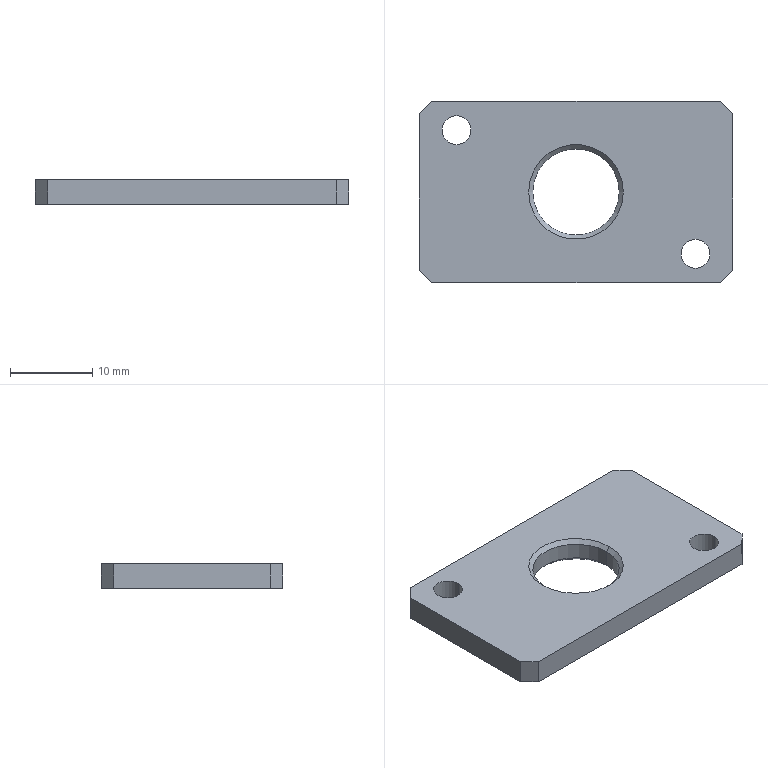Part | SolidWorks | features Chamfer 2, Extrusion 1 | 1 solid | 20 faces | box 38 x 22 x 3 mm | volume 2168 mm3 | plane 10 | cylinder 6 | cone 4 | commonest cylinder face diameters 3.5 x4 10.5 x2
STEP:
#1=CARTESIAN_POINT('',(-5.25,0.,2.5));
#2=VERTEX_POINT('',#1);
#3=CARTESIAN_POINT('',(5.25,0.,2.5));
#4=VERTEX_POINT('',#3);
#5=CARTESIAN_POINT('',(0.,0.,2.5));
#6=DIRECTION('',(0.,0.,1.));
#7=DIRECTION('',(1.,0.,0.));
#8=AXIS2_PLACEMENT_3D('',#5,#6,#7);
#9=CIRCLE('',#8,5.25);
#10=EDGE_CURVE('',#2,#4,#9,.T.);
#11=ORIENTED_EDGE('',*,*,#10,.F.);
#12=CARTESIAN_POINT('',(-5.75,0.,3.));
#13=VERTEX_POINT('',#12);
#14=CARTESIAN_POINT('',(-5.25,0.,2.5));
#15=DIRECTION('',(-0.7071,0.,0.7071));
#16=VECTOR('',#15,1000.);
#17=LINE('',#14,#16);
#18=EDGE_CURVE('',#2,#13,#17,.T.);
#19=ORIENTED_EDGE('',*,*,#18,.T.);
#20=CARTESIAN_POINT('',(5.75,0.,3.));
#21=VERTEX_POINT('',#20);
#22=CARTESIAN_POINT('',(0.,0.,3.));
#23=DIRECTION('',(0.,0.,-1.));
#24=DIRECTION('',(1.,0.,0.));
#25=AXIS2_PLACEMENT_3D('',#22,#23,#24);
#26=CIRCLE('',#25,5.75);
#27=EDGE_CURVE('',#21,#13,#26,.T.);
#28=ORIENTED_EDGE('',*,*,#27,.F.);
#29=CARTESIAN_POINT('',(5.25,0.,2.5));
#30=DIRECTION('',(0.7071,0.,0.7071));
#31=VECTOR('',#30,1000.);
#32=LINE('',#29,#31);
#33=EDGE_CURVE('',#4,#21,#32,.T.);
#34=ORIENTED_EDGE('',*,*,#33,.F.);
#35=EDGE_LOOP('',(#11,#19,#28,#34));
#36=FACE_OUTER_BOUND('',#35,.T.);
#37=CARTESIAN_POINT('',(0.,0.,2.5));
#38=DIRECTION('',(0.,0.,1.));
#39=DIRECTION('',(1.,0.,0.));
#40=AXIS2_PLACEMENT_3D('',#37,#38,#39);
#41=CONICAL_SURFACE('',#40,5.25,0.7854);
#42=ADVANCED_FACE('',(#36),#41,.F.);
#43=CARTESIAN_POINT('',(5.25,0.,0.5));
#44=VERTEX_POINT('',#43);
#45=CARTESIAN_POINT('',(-5.25,0.,0.5));
#46=VERTEX_POINT('',#45);
#47=CARTESIAN_POINT('',(0.,0.,0.5));
#48=DIRECTION('',(0.,0.,-1.));
#49=DIRECTION('',(1.,0.,0.));
#50=AXIS2_PLACEMENT_3D('',#47,#48,#49);
#51=CIRCLE('',#50,5.25);
#52=EDGE_CURVE('',#44,#46,#51,.T.);
#53=ORIENTED_EDGE('',*,*,#52,.F.);
#54=CARTESIAN_POINT('',(5.75,0.,0.));
#55=VERTEX_POINT('',#54);
#56=CARTESIAN_POINT('',(5.75,0.,0.));
#57=DIRECTION('',(0.7071,0.,-0.7071));
#58=VECTOR('',#57,1000.);
#59=LINE('',#56,#58);
#60=EDGE_CURVE('',#44,#55,#59,.T.);
#61=ORIENTED_EDGE('',*,*,#60,.T.);
#62=CARTESIAN_POINT('',(-5.75,0.,0.));
#63=VERTEX_POINT('',#62);
#64=CARTESIAN_POINT('',(0.,0.,0.));
#65=DIRECTION('',(0.,0.,1.));
#66=DIRECTION('',(1.,0.,0.));
#67=AXIS2_PLACEMENT_3D('',#64,#65,#66);
#68=CIRCLE('',#67,5.75);
#69=EDGE_CURVE('',#63,#55,#68,.T.);
#70=ORIENTED_EDGE('',*,*,#69,.F.);
#71=CARTESIAN_POINT('',(-5.75,0.,0.));
#72=DIRECTION('',(-0.7071,0.,-0.7071));
#73=VECTOR('',#72,1000.);
#74=LINE('',#71,#73);
#75=EDGE_CURVE('',#46,#63,#74,.T.);
#76=ORIENTED_EDGE('',*,*,#75,.F.);
#77=EDGE_LOOP('',(#53,#61,#70,#76));
#78=FACE_OUTER_BOUND('',#77,.T.);
#79=CARTESIAN_POINT('',(0.,0.,0.));
#80=DIRECTION('',(0.,0.,-1.));
#81=DIRECTION('',(-1.,0.,0.));
#82=AXIS2_PLACEMENT_3D('',#79,#80,#81);
#83=CONICAL_SURFACE('',#82,5.75,0.7854);
#84=ADVANCED_FACE('',(#78),#83,.F.);
#85=CARTESIAN_POINT('',(12.75,-7.5,3.));
#86=VERTEX_POINT('',#85);
#87=CARTESIAN_POINT('',(16.25,-7.5,3.));
#88=VERTEX_POINT('',#87);
#89=CARTESIAN_POINT('',(14.5,-7.5,3.));
#90=DIRECTION('',(0.,0.,1.));
#91=DIRECTION('',(1.,0.,0.));
#92=AXIS2_PLACEMENT_3D('',#89,#90,#91);
#93=CIRCLE('',#92,1.75);
#94=EDGE_CURVE('',#86,#88,#93,.T.);
#95=ORIENTED_EDGE('',*,*,#94,.T.);
#96=CARTESIAN_POINT('',(16.25,-7.5,0.));
#97=VERTEX_POINT('',#96);
#98=CARTESIAN_POINT('',(16.25,-7.5,3.));
#99=DIRECTION('',(0.,0.,-1.));
#100=VECTOR('',#99,1000.);
#101=LINE('',#98,#100);
#102=EDGE_CURVE('',#88,#97,#101,.T.);
#103=ORIENTED_EDGE('',*,*,#102,.T.);
#104=CARTESIAN_POINT('',(12.75,-7.5,0.));
#105=VERTEX_POINT('',#104);
#106=CARTESIAN_POINT('',(14.5,-7.5,0.));
#107=DIRECTION('',(0.,0.,1.));
#108=DIRECTION('',(1.,0.,0.));
#109=AXIS2_PLACEMENT_3D('',#106,#107,#108);
#110=CIRCLE('',#109,1.75);
#111=EDGE_CURVE('',#105,#97,#110,.T.);
#112=ORIENTED_EDGE('',*,*,#111,.F.);
#113=CARTESIAN_POINT('',(12.75,-7.5,3.));
#114=DIRECTION('',(0.,0.,-1.));
#115=VECTOR('',#114,1000.);
#116=LINE('',#113,#115);
#117=EDGE_CURVE('',#86,#105,#116,.T.);
#118=ORIENTED_EDGE('',*,*,#117,.F.);
#119=EDGE_LOOP('',(#95,#103,#112,#118));
#120=FACE_OUTER_BOUND('',#119,.T.);
#121=CARTESIAN_POINT('',(14.5,-7.5,3.));
#122=DIRECTION('',(0.,0.,-1.));
#123=DIRECTION('',(-1.,0.,0.));
#124=AXIS2_PLACEMENT_3D('',#121,#122,#123);
#125=CYLINDRICAL_SURFACE('',#124,1.75);
#126=ADVANCED_FACE('',(#120),#125,.F.);
#127=CARTESIAN_POINT('',(-16.25,7.5,3.));
#128=VERTEX_POINT('',#127);
#129=CARTESIAN_POINT('',(-12.75,7.5,3.));
#130=VERTEX_POINT('',#129);
#131=CARTESIAN_POINT('',(-14.5,7.5,3.));
#132=DIRECTION('',(0.,0.,1.));
#133=DIRECTION('',(1.,0.,0.));
#134=AXIS2_PLACEMENT_3D('',#131,#132,#133);
#135=CIRCLE('',#134,1.75);
#136=EDGE_CURVE('',#128,#130,#135,.T.);
#137=ORIENTED_EDGE('',*,*,#136,.T.);
#138=CARTESIAN_POINT('',(-12.75,7.5,0.));
#139=VERTEX_POINT('',#138);
#140=CARTESIAN_POINT('',(-12.75,7.5,3.));
#141=DIRECTION('',(0.,0.,-1.));
#142=VECTOR('',#141,1000.);
#143=LINE('',#140,#142);
#144=EDGE_CURVE('',#130,#139,#143,.T.);
#145=ORIENTED_EDGE('',*,*,#144,.T.);
#146=CARTESIAN_POINT('',(-16.25,7.5,0.));
#147=VERTEX_POINT('',#146);
#148=CARTESIAN_POINT('',(-14.5,7.5,0.));
#149=DIRECTION('',(0.,0.,1.));
#150=DIRECTION('',(1.,0.,0.));
#151=AXIS2_PLACEMENT_3D('',#148,#149,#150);
#152=CIRCLE('',#151,1.75);
#153=EDGE_CURVE('',#147,#139,#152,.T.);
#154=ORIENTED_EDGE('',*,*,#153,.F.);
#155=CARTESIAN_POINT('',(-16.25,7.5,3.));
#156=DIRECTION('',(0.,0.,-1.));
#157=VECTOR('',#156,1000.);
#158=LINE('',#155,#157);
#159=EDGE_CURVE('',#128,#147,#158,.T.);
#160=ORIENTED_EDGE('',*,*,#159,.F.);
#161=EDGE_LOOP('',(#137,#145,#154,#160));
#162=FACE_OUTER_BOUND('',#161,.T.);
#163=CARTESIAN_POINT('',(-14.5,7.5,3.));
#164=DIRECTION('',(0.,0.,-1.));
#165=DIRECTION('',(-1.,0.,0.));
#166=AXIS2_PLACEMENT_3D('',#163,#164,#165);
#167=CYLINDRICAL_SURFACE('',#166,1.75);
#168=ADVANCED_FACE('',(#162),#167,.F.);
#169=ORIENTED_EDGE('',*,*,#10,.T.);
#170=CARTESIAN_POINT('',(5.25,0.,3.));
#171=DIRECTION('',(0.,0.,-1.));
#172=VECTOR('',#171,1000.);
#173=LINE('',#170,#172);
#174=EDGE_CURVE('',#4,#44,#173,.T.);
#175=ORIENTED_EDGE('',*,*,#174,.T.);
#176=ORIENTED_EDGE('',*,*,#52,.T.);
#177=CARTESIAN_POINT('',(-5.25,0.,3.));
#178=DIRECTION('',(0.,0.,-1.));
#179=VECTOR('',#178,1000.);
#180=LINE('',#177,#179);
#181=EDGE_CURVE('',#2,#46,#180,.T.);
#182=ORIENTED_EDGE('',*,*,#181,.F.);
#183=EDGE_LOOP('',(#169,#175,#176,#182));
#184=FACE_OUTER_BOUND('',#183,.T.);
#185=CARTESIAN_POINT('',(0.,0.,3.));
#186=DIRECTION('',(0.,0.,-1.));
#187=DIRECTION('',(-1.,0.,0.));
#188=AXIS2_PLACEMENT_3D('',#185,#186,#187);
#189=CYLINDRICAL_SURFACE('',#188,5.25);
#190=ADVANCED_FACE('',(#184),#189,.F.);
#191=ORIENTED_EDGE('',*,*,#27,.T.);
#192=CARTESIAN_POINT('',(0.,0.,3.));
#193=DIRECTION('',(0.,0.,-1.));
#194=DIRECTION('',(1.,0.,0.));
#195=AXIS2_PLACEMENT_3D('',#192,#193,#194);
#196=CIRCLE('',#195,5.75);
#197=EDGE_CURVE('',#13,#21,#196,.T.);
#198=ORIENTED_EDGE('',*,*,#197,.T.);
#199=EDGE_LOOP('',(#191,#198));
#200=FACE_BOUND('',#199,.T.);
#201=ORIENTED_EDGE('',*,*,#136,.F.);
#202=CARTESIAN_POINT('',(-14.5,7.5,3.));
#203=DIRECTION('',(0.,0.,1.));
#204=DIRECTION('',(1.,0.,0.));
#205=AXIS2_PLACEMENT_3D('',#202,#203,#204);
#206=CIRCLE('',#205,1.75);
#207=EDGE_CURVE('',#130,#128,#206,.T.);
#208=ORIENTED_EDGE('',*,*,#207,.F.);
#209=EDGE_LOOP('',(#201,#208));
#210=FACE_BOUND('',#209,.T.);
#211=CARTESIAN_POINT('',(19.,-9.5,3.));
#212=VERTEX_POINT('',#211);
#213=CARTESIAN_POINT('',(19.,9.5,3.));
#214=VERTEX_POINT('',#213);
#215=CARTESIAN_POINT('',(19.,11.,3.));
#216=DIRECTION('',(0.,1.,0.));
#217=VECTOR('',#216,1000.);
#218=LINE('',#215,#217);
#219=EDGE_CURVE('',#212,#214,#218,.T.);
#220=ORIENTED_EDGE('',*,*,#219,.T.);
#221=CARTESIAN_POINT('',(17.5,11.,3.));
#222=VERTEX_POINT('',#221);
#223=CARTESIAN_POINT('',(29.25,-0.75,3.));
#224=DIRECTION('',(-0.7071,0.7071,0.));
#225=VECTOR('',#224,1000.);
#226=LINE('',#223,#225);
#227=EDGE_CURVE('',#214,#222,#226,.T.);
#228=ORIENTED_EDGE('',*,*,#227,.T.);
#229=CARTESIAN_POINT('',(-17.5,11.,3.));
#230=VERTEX_POINT('',#229);
#231=CARTESIAN_POINT('',(-19.,11.,3.));
#232=DIRECTION('',(-1.,0.,0.));
#233=VECTOR('',#232,1000.);
#234=LINE('',#231,#233);
#235=EDGE_CURVE('',#222,#230,#234,.T.);
#236=ORIENTED_EDGE('',*,*,#235,.T.);
#237=CARTESIAN_POINT('',(-19.,9.5,3.));
#238=VERTEX_POINT('',#237);
#239=CARTESIAN_POINT('',(-10.25,18.25,3.));
#240=DIRECTION('',(-0.7071,-0.7071,0.));
#241=VECTOR('',#240,1000.);
#242=LINE('',#239,#241);
#243=EDGE_CURVE('',#230,#238,#242,.T.);
#244=ORIENTED_EDGE('',*,*,#243,.T.);
#245=CARTESIAN_POINT('',(-19.,-9.5,3.));
#246=VERTEX_POINT('',#245);
#247=CARTESIAN_POINT('',(-19.,11.,3.));
#248=DIRECTION('',(0.,-1.,0.));
#249=VECTOR('',#248,1000.);
#250=LINE('',#247,#249);
#251=EDGE_CURVE('',#238,#246,#250,.T.);
#252=ORIENTED_EDGE('',*,*,#251,.T.);
#253=CARTESIAN_POINT('',(-17.5,-11.,3.));
#254=VERTEX_POINT('',#253);
#255=CARTESIAN_POINT('',(0.75,-29.25,3.));
#256=DIRECTION('',(0.7071,-0.7071,0.));
#257=VECTOR('',#256,1000.);
#258=LINE('',#255,#257);
#259=EDGE_CURVE('',#246,#254,#258,.T.);
#260=ORIENTED_EDGE('',*,*,#259,.T.);
#261=CARTESIAN_POINT('',(17.5,-11.,3.));
#262=VERTEX_POINT('',#261);
#263=CARTESIAN_POINT('',(-19.,-11.,3.));
#264=DIRECTION('',(1.,0.,0.));
#265=VECTOR('',#264,1000.);
#266=LINE('',#263,#265);
#267=EDGE_CURVE('',#254,#262,#266,.T.);
#268=ORIENTED_EDGE('',*,*,#267,.T.);
#269=CARTESIAN_POINT('',(18.25,-10.25,3.));
#270=DIRECTION('',(0.7071,0.7071,0.));
#271=VECTOR('',#270,1000.);
#272=LINE('',#269,#271);
#273=EDGE_CURVE('',#262,#212,#272,.T.);
#274=ORIENTED_EDGE('',*,*,#273,.T.);
#275=EDGE_LOOP('',(#220,#228,#236,#244,#252,#260,#268,#274));
#276=FACE_OUTER_BOUND('',#275,.T.);
#277=ORIENTED_EDGE('',*,*,#94,.F.);
#278=CARTESIAN_POINT('',(14.5,-7.5,3.));
#279=DIRECTION('',(0.,0.,1.));
#280=DIRECTION('',(1.,0.,0.));
#281=AXIS2_PLACEMENT_3D('',#278,#279,#280);
#282=CIRCLE('',#281,1.75);
#283=EDGE_CURVE('',#88,#86,#282,.T.);
#284=ORIENTED_EDGE('',*,*,#283,.F.);
#285=EDGE_LOOP('',(#277,#284));
#286=FACE_BOUND('',#285,.T.);
#287=CARTESIAN_POINT('',(19.,-11.,3.));
#288=DIRECTION('',(0.,0.,1.));
#289=DIRECTION('',(1.,0.,0.));
#290=AXIS2_PLACEMENT_3D('',#287,#288,#289);
#291=PLANE('',#290);
#292=ADVANCED_FACE('',(#200,#210,#276,#286),#291,.T.);
#293=ORIENTED_EDGE('',*,*,#69,.T.);
#294=CARTESIAN_POINT('',(0.,0.,0.));
#295=DIRECTION('',(0.,0.,1.));
#296=DIRECTION('',(1.,0.,0.));
#297=AXIS2_PLACEMENT_3D('',#294,#295,#296);
#298=CIRCLE('',#297,5.75);
#299=EDGE_CURVE('',#55,#63,#298,.T.);
#300=ORIENTED_EDGE('',*,*,#299,.T.);
#301=EDGE_LOOP('',(#293,#300));
#302=FACE_BOUND('',#301,.T.);
#303=ORIENTED_EDGE('',*,*,#153,.T.);
#304=CARTESIAN_POINT('',(-14.5,7.5,0.));
#305=DIRECTION('',(0.,0.,1.));
#306=DIRECTION('',(1.,0.,0.));
#307=AXIS2_PLACEMENT_3D('',#304,#305,#306);
#308=CIRCLE('',#307,1.75);
#309=EDGE_CURVE('',#139,#147,#308,.T.);
#310=ORIENTED_EDGE('',*,*,#309,.T.);
#311=EDGE_LOOP('',(#303,#310));
#312=FACE_BOUND('',#311,.T.);
#313=CARTESIAN_POINT('',(17.5,11.,0.));
#314=VERTEX_POINT('',#313);
#315=CARTESIAN_POINT('',(-17.5,11.,0.));
#316=VERTEX_POINT('',#315);
#317=CARTESIAN_POINT('',(-19.,11.,0.));
#318=DIRECTION('',(-1.,0.,0.));
#319=VECTOR('',#318,1000.);
#320=LINE('',#317,#319);
#321=EDGE_CURVE('',#314,#316,#320,.T.);
#322=ORIENTED_EDGE('',*,*,#321,.F.);
#323=CARTESIAN_POINT('',(19.,9.5,0.));
#324=VERTEX_POINT('',#323);
#325=CARTESIAN_POINT('',(17.5,11.,0.));
#326=DIRECTION('',(0.7071,-0.7071,0.));
#327=VECTOR('',#326,1000.);
#328=LINE('',#325,#327);
#329=EDGE_CURVE('',#314,#324,#328,.T.);
#330=ORIENTED_EDGE('',*,*,#329,.T.);
#331=CARTESIAN_POINT('',(19.,-9.5,0.));
#332=VERTEX_POINT('',#331);
#333=CARTESIAN_POINT('',(19.,11.,0.));
#334=DIRECTION('',(0.,1.,0.));
#335=VECTOR('',#334,1000.);
#336=LINE('',#333,#335);
#337=EDGE_CURVE('',#332,#324,#336,.T.);
#338=ORIENTED_EDGE('',*,*,#337,.F.);
#339=CARTESIAN_POINT('',(17.5,-11.,0.));
#340=VERTEX_POINT('',#339);
#341=CARTESIAN_POINT('',(19.,-9.5,0.));
#342=DIRECTION('',(-0.7071,-0.7071,0.));
#343=VECTOR('',#342,1000.);
#344=LINE('',#341,#343);
#345=EDGE_CURVE('',#332,#340,#344,.T.);
#346=ORIENTED_EDGE('',*,*,#345,.T.);
#347=CARTESIAN_POINT('',(-17.5,-11.,0.));
#348=VERTEX_POINT('',#347);
#349=CARTESIAN_POINT('',(-19.,-11.,0.));
#350=DIRECTION('',(1.,0.,0.));
#351=VECTOR('',#350,1000.);
#352=LINE('',#349,#351);
#353=EDGE_CURVE('',#348,#340,#352,.T.);
#354=ORIENTED_EDGE('',*,*,#353,.F.);
#355=CARTESIAN_POINT('',(-19.,-9.5,0.));
#356=VERTEX_POINT('',#355);
#357=CARTESIAN_POINT('',(-17.5,-11.,0.));
#358=DIRECTION('',(-0.7071,0.7071,0.));
#359=VECTOR('',#358,1000.);
#360=LINE('',#357,#359);
#361=EDGE_CURVE('',#348,#356,#360,.T.);
#362=ORIENTED_EDGE('',*,*,#361,.T.);
#363=CARTESIAN_POINT('',(-19.,9.5,0.));
#364=VERTEX_POINT('',#363);
#365=CARTESIAN_POINT('',(-19.,11.,0.));
#366=DIRECTION('',(0.,-1.,0.));
#367=VECTOR('',#366,1000.);
#368=LINE('',#365,#367);
#369=EDGE_CURVE('',#364,#356,#368,.T.);
#370=ORIENTED_EDGE('',*,*,#369,.F.);
#371=CARTESIAN_POINT('',(-19.,9.5,0.));
#372=DIRECTION('',(0.7071,0.7071,0.));
#373=VECTOR('',#372,1000.);
#374=LINE('',#371,#373);
#375=EDGE_CURVE('',#364,#316,#374,.T.);
#376=ORIENTED_EDGE('',*,*,#375,.T.);
#377=EDGE_LOOP('',(#322,#330,#338,#346,#354,#362,#370,#376));
#378=FACE_OUTER_BOUND('',#377,.T.);
#379=ORIENTED_EDGE('',*,*,#111,.T.);
#380=CARTESIAN_POINT('',(14.5,-7.5,0.));
#381=DIRECTION('',(0.,0.,1.));
#382=DIRECTION('',(1.,0.,0.));
#383=AXIS2_PLACEMENT_3D('',#380,#381,#382);
#384=CIRCLE('',#383,1.75);
#385=EDGE_CURVE('',#97,#105,#384,.T.);
#386=ORIENTED_EDGE('',*,*,#385,.T.);
#387=EDGE_LOOP('',(#379,#386));
#388=FACE_BOUND('',#387,.T.);
#389=CARTESIAN_POINT('',(19.,-11.,0.));
#390=DIRECTION('',(0.,0.,1.));
#391=DIRECTION('',(1.,0.,0.));
#392=AXIS2_PLACEMENT_3D('',#389,#390,#391);
#393=PLANE('',#392);
#394=ADVANCED_FACE('',(#302,#312,#378,#388),#393,.F.);
#395=ORIENTED_EDGE('',*,*,#337,.T.);
#396=CARTESIAN_POINT('',(19.,9.5,3.));
#397=DIRECTION('',(0.,0.,1.));
#398=VECTOR('',#397,1000.);
#399=LINE('',#396,#398);
#400=EDGE_CURVE('',#324,#214,#399,.T.);
#401=ORIENTED_EDGE('',*,*,#400,.T.);
#402=ORIENTED_EDGE('',*,*,#219,.F.);
#403=CARTESIAN_POINT('',(19.,-9.5,3.));
#404=DIRECTION('',(0.,0.,-1.));
#405=VECTOR('',#404,1000.);
#406=LINE('',#403,#405);
#407=EDGE_CURVE('',#212,#332,#406,.T.);
#408=ORIENTED_EDGE('',*,*,#407,.T.);
#409=EDGE_LOOP('',(#395,#401,#402,#408));
#410=FACE_OUTER_BOUND('',#409,.T.);
#411=CARTESIAN_POINT('',(19.,11.,3.));
#412=DIRECTION('',(-1.,0.,0.));
#413=DIRECTION('',(0.,-1.,0.));
#414=AXIS2_PLACEMENT_3D('',#411,#412,#413);
#415=PLANE('',#414);
#416=ADVANCED_FACE('',(#410),#415,.F.);
#417=ORIENTED_EDGE('',*,*,#235,.F.);
#418=CARTESIAN_POINT('',(17.5,11.,3.));
#419=DIRECTION('',(0.,0.,-1.));
#420=VECTOR('',#419,1000.);
#421=LINE('',#418,#420);
#422=EDGE_CURVE('',#222,#314,#421,.T.);
#423=ORIENTED_EDGE('',*,*,#422,.T.);
#424=ORIENTED_EDGE('',*,*,#321,.T.);
#425=CARTESIAN_POINT('',(-17.5,11.,3.));
#426=DIRECTION('',(0.,0.,1.));
#427=VECTOR('',#426,1000.);
#428=LINE('',#425,#427);
#429=EDGE_CURVE('',#316,#230,#428,.T.);
#430=ORIENTED_EDGE('',*,*,#429,.T.);
#431=EDGE_LOOP('',(#417,#423,#424,#430));
#432=FACE_OUTER_BOUND('',#431,.T.);
#433=CARTESIAN_POINT('',(-19.,11.,3.));
#434=DIRECTION('',(0.,-1.,0.));
#435=DIRECTION('',(0.,0.,-1.));
#436=AXIS2_PLACEMENT_3D('',#433,#434,#435);
#437=PLANE('',#436);
#438=ADVANCED_FACE('',(#432),#437,.F.);
#439=ORIENTED_EDGE('',*,*,#369,.T.);
#440=CARTESIAN_POINT('',(-19.,-9.5,3.));
#441=DIRECTION('',(0.,0.,1.));
#442=VECTOR('',#441,1000.);
#443=LINE('',#440,#442);
#444=EDGE_CURVE('',#356,#246,#443,.T.);
#445=ORIENTED_EDGE('',*,*,#444,.T.);
#446=ORIENTED_EDGE('',*,*,#251,.F.);
#447=CARTESIAN_POINT('',(-19.,9.5,3.));
#448=DIRECTION('',(0.,0.,-1.));
#449=VECTOR('',#448,1000.);
#450=LINE('',#447,#449);
#451=EDGE_CURVE('',#238,#364,#450,.T.);
#452=ORIENTED_EDGE('',*,*,#451,.T.);
#453=EDGE_LOOP('',(#439,#445,#446,#452));
#454=FACE_OUTER_BOUND('',#453,.T.);
#455=CARTESIAN_POINT('',(-19.,11.,3.));
#456=DIRECTION('',(1.,0.,0.));
#457=DIRECTION('',(0.,0.,-1.));
#458=AXIS2_PLACEMENT_3D('',#455,#456,#457);
#459=PLANE('',#458);
#460=ADVANCED_FACE('',(#454),#459,.F.);
#461=ORIENTED_EDGE('',*,*,#353,.T.);
#462=CARTESIAN_POINT('',(17.5,-11.,3.));
#463=DIRECTION('',(0.,0.,1.));
#464=VECTOR('',#463,1000.);
#465=LINE('',#462,#464);
#466=EDGE_CURVE('',#340,#262,#465,.T.);
#467=ORIENTED_EDGE('',*,*,#466,.T.);
#468=ORIENTED_EDGE('',*,*,#267,.F.);
#469=CARTESIAN_POINT('',(-17.5,-11.,3.));
#470=DIRECTION('',(0.,0.,-1.));
#471=VECTOR('',#470,1000.);
#472=LINE('',#469,#471);
#473=EDGE_CURVE('',#254,#348,#472,.T.);
#474=ORIENTED_EDGE('',*,*,#473,.T.);
#475=EDGE_LOOP('',(#461,#467,#468,#474));
#476=FACE_OUTER_BOUND('',#475,.T.);
#477=CARTESIAN_POINT('',(-19.,-11.,3.));
#478=DIRECTION('',(0.,1.,0.));
#479=DIRECTION('',(0.,0.,1.));
#480=AXIS2_PLACEMENT_3D('',#477,#478,#479);
#481=PLANE('',#480);
#482=ADVANCED_FACE('',(#476),#481,.F.);
#483=ORIENTED_EDGE('',*,*,#174,.F.);
#484=CARTESIAN_POINT('',(0.,0.,2.5));
#485=DIRECTION('',(0.,0.,1.));
#486=DIRECTION('',(1.,0.,0.));
#487=AXIS2_PLACEMENT_3D('',#484,#485,#486);
#488=CIRCLE('',#487,5.25);
#489=EDGE_CURVE('',#4,#2,#488,.T.);
#490=ORIENTED_EDGE('',*,*,#489,.T.);
#491=ORIENTED_EDGE('',*,*,#181,.T.);
#492=CARTESIAN_POINT('',(0.,0.,0.5));
#493=DIRECTION('',(0.,0.,-1.));
#494=DIRECTION('',(1.,0.,0.));
#495=AXIS2_PLACEMENT_3D('',#492,#493,#494);
#496=CIRCLE('',#495,5.25);
#497=EDGE_CURVE('',#46,#44,#496,.T.);
#498=ORIENTED_EDGE('',*,*,#497,.T.);
#499=EDGE_LOOP('',(#483,#490,#491,#498));
#500=FACE_OUTER_BOUND('',#499,.T.);
#501=CARTESIAN_POINT('',(0.,0.,3.));
#502=DIRECTION('',(0.,0.,-1.));
#503=DIRECTION('',(-1.,0.,0.));
#504=AXIS2_PLACEMENT_3D('',#501,#502,#503);
#505=CYLINDRICAL_SURFACE('',#504,5.25);
#506=ADVANCED_FACE('',(#500),#505,.F.);
#507=ORIENTED_EDGE('',*,*,#144,.F.);
#508=ORIENTED_EDGE('',*,*,#207,.T.);
#509=ORIENTED_EDGE('',*,*,#159,.T.);
#510=ORIENTED_EDGE('',*,*,#309,.F.);
#511=EDGE_LOOP('',(#507,#508,#509,#510));
#512=FACE_OUTER_BOUND('',#511,.T.);
#513=CARTESIAN_POINT('',(-14.5,7.5,3.));
#514=DIRECTION('',(0.,0.,-1.));
#515=DIRECTION('',(-1.,0.,0.));
#516=AXIS2_PLACEMENT_3D('',#513,#514,#515);
#517=CYLINDRICAL_SURFACE('',#516,1.75);
#518=ADVANCED_FACE('',(#512),#517,.F.);
#519=ORIENTED_EDGE('',*,*,#102,.F.);
#520=ORIENTED_EDGE('',*,*,#283,.T.);
#521=ORIENTED_EDGE('',*,*,#117,.T.);
#522=ORIENTED_EDGE('',*,*,#385,.F.);
#523=EDGE_LOOP('',(#519,#520,#521,#522));
#524=FACE_OUTER_BOUND('',#523,.T.);
#525=CARTESIAN_POINT('',(14.5,-7.5,3.));
#526=DIRECTION('',(0.,0.,-1.));
#527=DIRECTION('',(-1.,0.,0.));
#528=AXIS2_PLACEMENT_3D('',#525,#526,#527);
#529=CYLINDRICAL_SURFACE('',#528,1.75);
#530=ADVANCED_FACE('',(#524),#529,.F.);
#531=ORIENTED_EDGE('',*,*,#227,.F.);
#532=ORIENTED_EDGE('',*,*,#400,.F.);
#533=ORIENTED_EDGE('',*,*,#329,.F.);
#534=ORIENTED_EDGE('',*,*,#422,.F.);
#535=EDGE_LOOP('',(#531,#532,#533,#534));
#536=FACE_OUTER_BOUND('',#535,.T.);
#537=CARTESIAN_POINT('',(17.5,11.,3.));
#538=DIRECTION('',(-0.7071,-0.7071,0.));
#539=DIRECTION('',(0.7071,-0.7071,0.));
#540=AXIS2_PLACEMENT_3D('',#537,#538,#539);
#541=PLANE('',#540);
#542=ADVANCED_FACE('',(#536),#541,.F.);
#543=ORIENTED_EDGE('',*,*,#273,.F.);
#544=ORIENTED_EDGE('',*,*,#466,.F.);
#545=ORIENTED_EDGE('',*,*,#345,.F.);
#546=ORIENTED_EDGE('',*,*,#407,.F.);
#547=EDGE_LOOP('',(#543,#544,#545,#546));
#548=FACE_OUTER_BOUND('',#547,.T.);
#549=CARTESIAN_POINT('',(19.,-9.5,3.));
#550=DIRECTION('',(-0.7071,0.7071,0.));
#551=DIRECTION('',(-0.7071,-0.7071,0.));
#552=AXIS2_PLACEMENT_3D('',#549,#550,#551);
#553=PLANE('',#552);
#554=ADVANCED_FACE('',(#548),#553,.F.);
#555=ORIENTED_EDGE('',*,*,#259,.F.);
#556=ORIENTED_EDGE('',*,*,#444,.F.);
#557=ORIENTED_EDGE('',*,*,#361,.F.);
#558=ORIENTED_EDGE('',*,*,#473,.F.);
#559=EDGE_LOOP('',(#555,#556,#557,#558));
#560=FACE_OUTER_BOUND('',#559,.T.);
#561=CARTESIAN_POINT('',(-17.5,-11.,3.));
#562=DIRECTION('',(0.7071,0.7071,0.));
#563=DIRECTION('',(-0.7071,0.7071,0.));
#564=AXIS2_PLACEMENT_3D('',#561,#562,#563);
#565=PLANE('',#564);
#566=ADVANCED_FACE('',(#560),#565,.F.);
#567=ORIENTED_EDGE('',*,*,#243,.F.);
#568=ORIENTED_EDGE('',*,*,#429,.F.);
#569=ORIENTED_EDGE('',*,*,#375,.F.);
#570=ORIENTED_EDGE('',*,*,#451,.F.);
#571=EDGE_LOOP('',(#567,#568,#569,#570));
#572=FACE_OUTER_BOUND('',#571,.T.);
#573=CARTESIAN_POINT('',(-19.,9.5,3.));
#574=DIRECTION('',(0.7071,-0.7071,0.));
#575=DIRECTION('',(0.7071,0.7071,0.));
#576=AXIS2_PLACEMENT_3D('',#573,#574,#575);
#577=PLANE('',#576);
#578=ADVANCED_FACE('',(#572),#577,.F.);
#579=ORIENTED_EDGE('',*,*,#60,.F.);
#580=ORIENTED_EDGE('',*,*,#497,.F.);
#581=ORIENTED_EDGE('',*,*,#75,.T.);
#582=ORIENTED_EDGE('',*,*,#299,.F.);
#583=EDGE_LOOP('',(#579,#580,#581,#582));
#584=FACE_OUTER_BOUND('',#583,.T.);
#585=CARTESIAN_POINT('',(0.,0.,0.));
#586=DIRECTION('',(0.,0.,-1.));
#587=DIRECTION('',(-1.,0.,0.));
#588=AXIS2_PLACEMENT_3D('',#585,#586,#587);
#589=CONICAL_SURFACE('',#588,5.75,0.7854);
#590=ADVANCED_FACE('',(#584),#589,.F.);
#591=ORIENTED_EDGE('',*,*,#18,.F.);
#592=ORIENTED_EDGE('',*,*,#489,.F.);
#593=ORIENTED_EDGE('',*,*,#33,.T.);
#594=ORIENTED_EDGE('',*,*,#197,.F.);
#595=EDGE_LOOP('',(#591,#592,#593,#594));
#596=FACE_OUTER_BOUND('',#595,.T.);
#597=CARTESIAN_POINT('',(0.,0.,2.5));
#598=DIRECTION('',(0.,0.,1.));
#599=DIRECTION('',(1.,0.,0.));
#600=AXIS2_PLACEMENT_3D('',#597,#598,#599);
#601=CONICAL_SURFACE('',#600,5.25,0.7854);
#602=ADVANCED_FACE('',(#596),#601,.F.);
#603=CLOSED_SHELL('',(#42,#84,#126,#168,#190,#292,#394,#416,#438,#460,#482,#506,#518,#530,#542,#554,#566,#578,#590,#602));
#604=MANIFOLD_SOLID_BREP('',#603);
#605=CARTESIAN_POINT('',(0.,0.,0.));
#606=DIRECTION('',(0.,0.,1.));
#607=DIRECTION('',(1.,0.,0.));
#608=AXIS2_PLACEMENT_3D('',#605,#606,#607);
#609=(LENGTH_UNIT()NAMED_UNIT(*)SI_UNIT(.MILLI.,.METRE.));
#610=UNCERTAINTY_MEASURE_WITH_UNIT(LENGTH_MEASURE(0.00001),#609,'','');
#611=(NAMED_UNIT(*)PLANE_ANGLE_UNIT()SI_UNIT($,.RADIAN.));
#612=(NAMED_UNIT(*)SI_UNIT($,.STERADIAN.)SOLID_ANGLE_UNIT());
#613=(GEOMETRIC_REPRESENTATION_CONTEXT(3)GLOBAL_UNCERTAINTY_ASSIGNED_CONTEXT((#610))GLOBAL_UNIT_ASSIGNED_CONTEXT((#609,#611,#612))REPRESENTATION_CONTEXT('',''));
#614=ADVANCED_BREP_SHAPE_REPRESENTATION('',(#604,#608),#613);